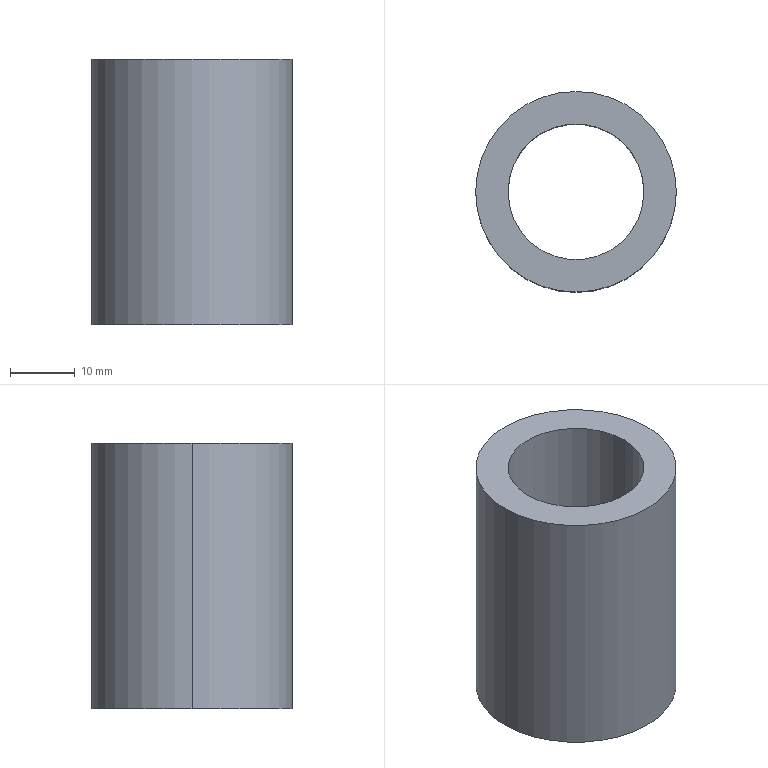Part | SolidWorks | features Extrusion 1 | 1 solid | 6 faces | box 31 x 31 x 41 mm | volume 16745 mm3 | cylinder 4 | plane 2 | commonest cylinder face diameters 21 x2 31 x2
STEP:
#1=CARTESIAN_POINT('',(-10.5,0.,41.));
#2=VERTEX_POINT('',#1);
#3=CARTESIAN_POINT('',(10.5,0.,41.));
#4=VERTEX_POINT('',#3);
#5=CARTESIAN_POINT('',(0.,0.,41.));
#6=DIRECTION('',(0.,0.,1.));
#7=DIRECTION('',(1.,0.,0.));
#8=AXIS2_PLACEMENT_3D('',#5,#6,#7);
#9=CIRCLE('',#8,10.5);
#10=EDGE_CURVE('',#2,#4,#9,.T.);
#11=ORIENTED_EDGE('',*,*,#10,.T.);
#12=CARTESIAN_POINT('',(10.5,0.,0.));
#13=VERTEX_POINT('',#12);
#14=CARTESIAN_POINT('',(10.5,0.,41.));
#15=DIRECTION('',(0.,0.,-1.));
#16=VECTOR('',#15,1000.);
#17=LINE('',#14,#16);
#18=EDGE_CURVE('',#4,#13,#17,.T.);
#19=ORIENTED_EDGE('',*,*,#18,.T.);
#20=CARTESIAN_POINT('',(-10.5,0.,0.));
#21=VERTEX_POINT('',#20);
#22=CARTESIAN_POINT('',(0.,0.,0.));
#23=DIRECTION('',(0.,0.,1.));
#24=DIRECTION('',(1.,0.,0.));
#25=AXIS2_PLACEMENT_3D('',#22,#23,#24);
#26=CIRCLE('',#25,10.5);
#27=EDGE_CURVE('',#21,#13,#26,.T.);
#28=ORIENTED_EDGE('',*,*,#27,.F.);
#29=CARTESIAN_POINT('',(-10.5,0.,41.));
#30=DIRECTION('',(0.,0.,-1.));
#31=VECTOR('',#30,1000.);
#32=LINE('',#29,#31);
#33=EDGE_CURVE('',#2,#21,#32,.T.);
#34=ORIENTED_EDGE('',*,*,#33,.F.);
#35=EDGE_LOOP('',(#11,#19,#28,#34));
#36=FACE_OUTER_BOUND('',#35,.T.);
#37=CARTESIAN_POINT('',(0.,0.,41.));
#38=DIRECTION('',(0.,0.,-1.));
#39=DIRECTION('',(-1.,0.,0.));
#40=AXIS2_PLACEMENT_3D('',#37,#38,#39);
#41=CYLINDRICAL_SURFACE('',#40,10.5);
#42=ADVANCED_FACE('',(#36),#41,.F.);
#43=CARTESIAN_POINT('',(15.5,0.,41.));
#44=VERTEX_POINT('',#43);
#45=CARTESIAN_POINT('',(-15.5,0.,41.));
#46=VERTEX_POINT('',#45);
#47=CARTESIAN_POINT('',(0.,0.,41.));
#48=DIRECTION('',(0.,0.,1.));
#49=DIRECTION('',(1.,0.,0.));
#50=AXIS2_PLACEMENT_3D('',#47,#48,#49);
#51=CIRCLE('',#50,15.5);
#52=EDGE_CURVE('',#44,#46,#51,.T.);
#53=ORIENTED_EDGE('',*,*,#52,.F.);
#54=CARTESIAN_POINT('',(15.5,0.,0.));
#55=VERTEX_POINT('',#54);
#56=CARTESIAN_POINT('',(15.5,0.,41.));
#57=DIRECTION('',(0.,0.,-1.));
#58=VECTOR('',#57,1000.);
#59=LINE('',#56,#58);
#60=EDGE_CURVE('',#44,#55,#59,.T.);
#61=ORIENTED_EDGE('',*,*,#60,.T.);
#62=CARTESIAN_POINT('',(-15.5,0.,0.));
#63=VERTEX_POINT('',#62);
#64=CARTESIAN_POINT('',(0.,0.,0.));
#65=DIRECTION('',(0.,0.,1.));
#66=DIRECTION('',(1.,0.,0.));
#67=AXIS2_PLACEMENT_3D('',#64,#65,#66);
#68=CIRCLE('',#67,15.5);
#69=EDGE_CURVE('',#55,#63,#68,.T.);
#70=ORIENTED_EDGE('',*,*,#69,.T.);
#71=CARTESIAN_POINT('',(-15.5,0.,41.));
#72=DIRECTION('',(0.,0.,-1.));
#73=VECTOR('',#72,1000.);
#74=LINE('',#71,#73);
#75=EDGE_CURVE('',#46,#63,#74,.T.);
#76=ORIENTED_EDGE('',*,*,#75,.F.);
#77=EDGE_LOOP('',(#53,#61,#70,#76));
#78=FACE_OUTER_BOUND('',#77,.T.);
#79=CARTESIAN_POINT('',(0.,0.,41.));
#80=DIRECTION('',(0.,0.,-1.));
#81=DIRECTION('',(-1.,0.,0.));
#82=AXIS2_PLACEMENT_3D('',#79,#80,#81);
#83=CYLINDRICAL_SURFACE('',#82,15.5);
#84=ADVANCED_FACE('',(#78),#83,.T.);
#85=CARTESIAN_POINT('',(0.,0.,41.));
#86=DIRECTION('',(0.,0.,1.));
#87=DIRECTION('',(1.,0.,0.));
#88=AXIS2_PLACEMENT_3D('',#85,#86,#87);
#89=CIRCLE('',#88,15.5);
#90=EDGE_CURVE('',#46,#44,#89,.T.);
#91=ORIENTED_EDGE('',*,*,#90,.T.);
#92=ORIENTED_EDGE('',*,*,#52,.T.);
#93=EDGE_LOOP('',(#91,#92));
#94=FACE_OUTER_BOUND('',#93,.T.);
#95=ORIENTED_EDGE('',*,*,#10,.F.);
#96=CARTESIAN_POINT('',(0.,0.,41.));
#97=DIRECTION('',(0.,0.,1.));
#98=DIRECTION('',(1.,0.,0.));
#99=AXIS2_PLACEMENT_3D('',#96,#97,#98);
#100=CIRCLE('',#99,10.5);
#101=EDGE_CURVE('',#4,#2,#100,.T.);
#102=ORIENTED_EDGE('',*,*,#101,.F.);
#103=EDGE_LOOP('',(#95,#102));
#104=FACE_BOUND('',#103,.T.);
#105=CARTESIAN_POINT('',(0.,0.,41.));
#106=DIRECTION('',(0.,0.,1.));
#107=DIRECTION('',(1.,0.,0.));
#108=AXIS2_PLACEMENT_3D('',#105,#106,#107);
#109=PLANE('',#108);
#110=ADVANCED_FACE('',(#94,#104),#109,.T.);
#111=CARTESIAN_POINT('',(0.,0.,0.));
#112=DIRECTION('',(0.,0.,1.));
#113=DIRECTION('',(1.,0.,0.));
#114=AXIS2_PLACEMENT_3D('',#111,#112,#113);
#115=CIRCLE('',#114,15.5);
#116=EDGE_CURVE('',#63,#55,#115,.T.);
#117=ORIENTED_EDGE('',*,*,#116,.F.);
#118=ORIENTED_EDGE('',*,*,#69,.F.);
#119=EDGE_LOOP('',(#117,#118));
#120=FACE_OUTER_BOUND('',#119,.T.);
#121=ORIENTED_EDGE('',*,*,#27,.T.);
#122=CARTESIAN_POINT('',(0.,0.,0.));
#123=DIRECTION('',(0.,0.,1.));
#124=DIRECTION('',(1.,0.,0.));
#125=AXIS2_PLACEMENT_3D('',#122,#123,#124);
#126=CIRCLE('',#125,10.5);
#127=EDGE_CURVE('',#13,#21,#126,.T.);
#128=ORIENTED_EDGE('',*,*,#127,.T.);
#129=EDGE_LOOP('',(#121,#128));
#130=FACE_BOUND('',#129,.T.);
#131=CARTESIAN_POINT('',(0.,0.,0.));
#132=DIRECTION('',(0.,0.,1.));
#133=DIRECTION('',(1.,0.,0.));
#134=AXIS2_PLACEMENT_3D('',#131,#132,#133);
#135=PLANE('',#134);
#136=ADVANCED_FACE('',(#120,#130),#135,.F.);
#137=ORIENTED_EDGE('',*,*,#60,.F.);
#138=ORIENTED_EDGE('',*,*,#90,.F.);
#139=ORIENTED_EDGE('',*,*,#75,.T.);
#140=ORIENTED_EDGE('',*,*,#116,.T.);
#141=EDGE_LOOP('',(#137,#138,#139,#140));
#142=FACE_OUTER_BOUND('',#141,.T.);
#143=CARTESIAN_POINT('',(0.,0.,41.));
#144=DIRECTION('',(0.,0.,-1.));
#145=DIRECTION('',(-1.,0.,0.));
#146=AXIS2_PLACEMENT_3D('',#143,#144,#145);
#147=CYLINDRICAL_SURFACE('',#146,15.5);
#148=ADVANCED_FACE('',(#142),#147,.T.);
#149=ORIENTED_EDGE('',*,*,#18,.F.);
#150=ORIENTED_EDGE('',*,*,#101,.T.);
#151=ORIENTED_EDGE('',*,*,#33,.T.);
#152=ORIENTED_EDGE('',*,*,#127,.F.);
#153=EDGE_LOOP('',(#149,#150,#151,#152));
#154=FACE_OUTER_BOUND('',#153,.T.);
#155=CARTESIAN_POINT('',(0.,0.,41.));
#156=DIRECTION('',(0.,0.,-1.));
#157=DIRECTION('',(-1.,0.,0.));
#158=AXIS2_PLACEMENT_3D('',#155,#156,#157);
#159=CYLINDRICAL_SURFACE('',#158,10.5);
#160=ADVANCED_FACE('',(#154),#159,.F.);
#161=CLOSED_SHELL('',(#42,#84,#110,#136,#148,#160));
#162=MANIFOLD_SOLID_BREP('',#161);
#163=CARTESIAN_POINT('',(0.,0.,0.));
#164=DIRECTION('',(0.,0.,1.));
#165=DIRECTION('',(1.,0.,0.));
#166=AXIS2_PLACEMENT_3D('',#163,#164,#165);
#167=(LENGTH_UNIT()NAMED_UNIT(*)SI_UNIT(.MILLI.,.METRE.));
#168=UNCERTAINTY_MEASURE_WITH_UNIT(LENGTH_MEASURE(0.00001),#167,'','');
#169=(NAMED_UNIT(*)PLANE_ANGLE_UNIT()SI_UNIT($,.RADIAN.));
#170=(NAMED_UNIT(*)SI_UNIT($,.STERADIAN.)SOLID_ANGLE_UNIT());
#171=(GEOMETRIC_REPRESENTATION_CONTEXT(3)GLOBAL_UNCERTAINTY_ASSIGNED_CONTEXT((#168))GLOBAL_UNIT_ASSIGNED_CONTEXT((#167,#169,#170))REPRESENTATION_CONTEXT('',''));
#172=ADVANCED_BREP_SHAPE_REPRESENTATION('',(#162,#166),#171);